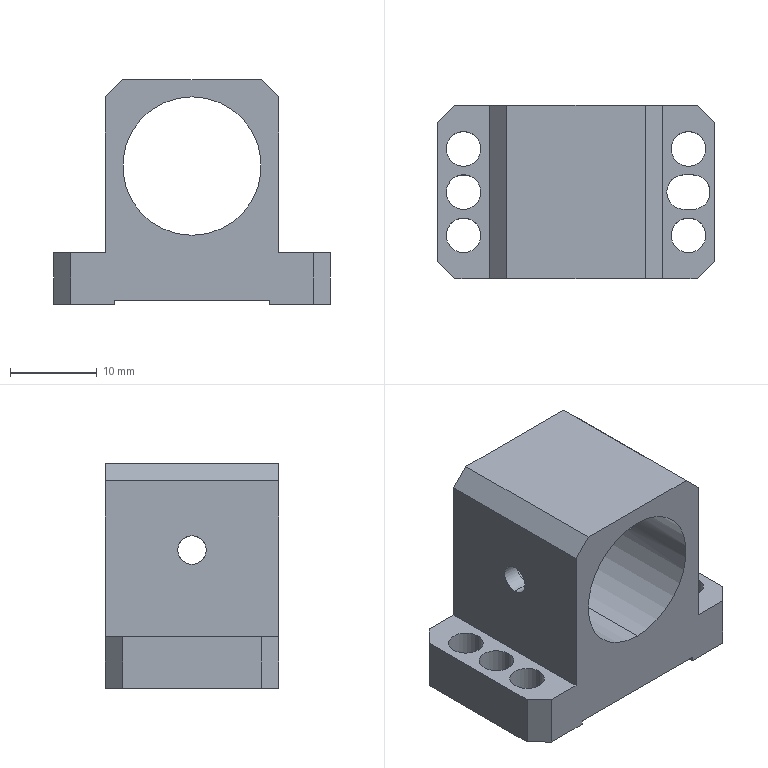NC program | NX | posted with a generic post | part box 32 x 20 x 26 mm
Lines 1 to 2179 of 2593, first 1714 of 2167 lines:
N10 G17 G21 G94 G90
(FLOOR_WALL , TOOL : D10JING)
N12 T11 M6
N14 G54
N16 G17 G0 G90 X-17.997 Y-20. B0. C0. S9500 M3
N18 G43 Z30. H11
N20 Z3.
N22 G94 G1 Z0. F1250.
N24 Y-17.
N26 Y17.
N28 X-13.426
N30 Y-17.
N32 X-8.855
N34 Y17.
N36 X-4.284
N38 Y-17.
N40 X0.287
N42 Y17.
N44 X4.858
N46 Y-17.
N48 X9.429
N50 Y17.
N52 X14.
N54 Y-17.
N56 Y-20.
N58 Z3.
N60 G0 Z30.
N62 M5
(ZLEVEL_PROFILE , TOOL : D10)
N64 T10 M6
N66 G54
N68 G17 G0 G90 X13.531 Y15.1 B0. C0. S9500 M3
N70 G43 Z30. H10
N72 Z1.5
N74 G94 G1 X14.32 Z1.459 F1000.
N76 X15.153 Y14.978 Z1.415
N78 X15.956 Y14.721 Z1.37
N80 X16.705 Y14.336 Z1.326
N82 X17.38 Y13.832 Z1.282
N84 X19.832 Y11.38 Z1.1
N86 X20.336 Y10.705 Z1.056
N88 X20.721 Y9.956 Z1.012
N90 X20.978 Y9.153 Z0.968
N92 X21.1 Y8.32 Z0.924
N94 Y-8.32 Z0.052
N96 X20.978 Y-9.153 Z0.008
N98 X20.721 Y-9.956 Z-0.037
N100 X20.336 Y-10.705 Z-0.081
N102 X19.832 Y-11.38 Z-0.125
N104 X17.38 Y-13.832 Z-0.307
N106 X16.705 Y-14.336 Z-0.351
N108 X15.956 Y-14.721 Z-0.395
N110 X15.153 Y-14.978 Z-0.439
N112 X14.32 Y-15.1 Z-0.483
N114 X14. Z-0.5
N116 X-14. F3000.
N118 G2 X-17.606 Y-13.606 R5.1
N120 G1 X-19.606 Y-11.606
N122 G2 X-21.1 Y-8. R5.1
N124 G1 Y8.
N126 G2 X-19.606 Y11.606 R5.1
N128 G1 X-17.606 Y13.606
N130 G2 X-14. Y15.1 R5.1
N132 G1 X14.
N134 G2 X17.606 Y13.606 R5.1
N136 G1 X19.606 Y11.606
N138 G2 X21.1 Y8. R5.1
N140 G1 Y-8.
N142 G2 X19.606 Y-11.606 R5.1
N144 G1 X17.606 Y-13.606
N146 G2 X14. Y-15.1 R5.1
N148 G1 X-13.764 Z-0.985
N150 X-13.984 Z-0.988
N152 X-14.204 Y-15.096 Z-0.992
N154 X-14.424 Y-15.082 Z-0.996
N156 X-14.643 Y-15.059 Z-1.
N158 G2 X-17.606 Y-13.606 R5.1
N160 G1 X-19.606 Y-11.606
N162 G2 X-21.1 Y-8. R5.1
N164 G1 Y8.
N166 G2 X-19.606 Y11.606 R5.1
N168 G1 X-17.606 Y13.606
N170 G2 X-14. Y15.1 R5.1
N172 G1 X14.
N174 G2 X17.606 Y13.606 R5.1
N176 G1 X19.606 Y11.606
N178 G2 X21.1 Y8. R5.1
N180 G1 Y-8.
N182 G2 X19.606 Y-11.606 R5.1
N184 G1 X17.606 Y-13.606
N186 G2 X14. Y-15.1 R5.1
N188 G1 X-13.764 Z-1.485
N190 X-13.984 Z-1.488
N192 X-14.204 Y-15.096 Z-1.492
N194 X-14.424 Y-15.082 Z-1.496
N196 X-14.643 Y-15.059 Z-1.5
N198 G2 X-17.606 Y-13.606 R5.1
N200 G1 X-19.606 Y-11.606
N202 G2 X-21.1 Y-8. R5.1
N204 G1 Y8.
N206 G2 X-19.606 Y11.606 R5.1
N208 G1 X-17.606 Y13.606
N210 G2 X-14. Y15.1 R5.1
N212 G1 X14.
N214 G2 X17.606 Y13.606 R5.1
N216 G1 X19.606 Y11.606
N218 G2 X21.1 Y8. R5.1
N220 G1 Y-8.
N222 G2 X19.606 Y-11.606 R5.1
N224 G1 X17.606 Y-13.606
N226 G2 X14. Y-15.1 R5.1
N228 G1 X-13.764 Z-1.985
N230 X-13.984 Z-1.988
N232 X-14.204 Y-15.096 Z-1.992
N234 X-14.424 Y-15.082 Z-1.996
N236 X-14.643 Y-15.059 Z-2.
N238 G2 X-17.606 Y-13.606 R5.1
N240 G1 X-19.606 Y-11.606
N242 G2 X-21.1 Y-8. R5.1
N244 G1 Y8.
N246 G2 X-19.606 Y11.606 R5.1
N248 G1 X-17.606 Y13.606
N250 G2 X-14. Y15.1 R5.1
N252 G1 X14.
N254 G2 X17.606 Y13.606 R5.1
N256 G1 X19.606 Y11.606
N258 G2 X21.1 Y8. R5.1
N260 G1 Y-8.
N262 G2 X19.606 Y-11.606 R5.1
N264 G1 X17.606 Y-13.606
N266 G2 X14. Y-15.1 R5.1
N268 G1 X-13.764 Z-2.485
N270 X-13.984 Z-2.488
N272 X-14.204 Y-15.096 Z-2.492
N274 X-14.424 Y-15.082 Z-2.496
N276 X-14.643 Y-15.059 Z-2.5
N278 G2 X-17.606 Y-13.606 R5.1
N280 G1 X-19.606 Y-11.606
N282 G2 X-21.1 Y-8. R5.1
N284 G1 Y8.
N286 G2 X-19.606 Y11.606 R5.1
N288 G1 X-17.606 Y13.606
N290 G2 X-14. Y15.1 R5.1
N292 G1 X14.
N294 G2 X17.606 Y13.606 R5.1
N296 G1 X19.606 Y11.606
N298 G2 X21.1 Y8. R5.1
N300 G1 Y-8.
N302 G2 X19.606 Y-11.606 R5.1
N304 G1 X17.606 Y-13.606
N306 G2 X14. Y-15.1 R5.1
N308 G1 X-13.764 Z-2.985
N310 X-13.984 Z-2.988
N312 X-14.204 Y-15.096 Z-2.992
N314 X-14.424 Y-15.082 Z-2.996
N316 X-14.643 Y-15.059 Z-3.
N318 G2 X-17.606 Y-13.606 R5.1
N320 G1 X-19.606 Y-11.606
N322 G2 X-21.1 Y-8. R5.1
N324 G1 Y8.
N326 G2 X-19.606 Y11.606 R5.1
N328 G1 X-17.606 Y13.606
N330 G2 X-14. Y15.1 R5.1
N332 G1 X14.
N334 G2 X17.606 Y13.606 R5.1
N336 G1 X19.606 Y11.606
N338 G2 X21.1 Y8. R5.1
N340 G1 Y-8.
N342 G2 X19.606 Y-11.606 R5.1
N344 G1 X17.606 Y-13.606
N346 G2 X14. Y-15.1 R5.1
N348 G1 X-13.764 Z-3.485
N350 X-13.984 Z-3.488
N352 X-14.204 Y-15.096 Z-3.492
N354 X-14.424 Y-15.082 Z-3.496
N356 X-14.643 Y-15.059 Z-3.5
N358 G2 X-17.606 Y-13.606 R5.1
N360 G1 X-19.606 Y-11.606
N362 G2 X-21.1 Y-8. R5.1
N364 G1 Y8.
N366 G2 X-19.606 Y11.606 R5.1
N368 G1 X-17.606 Y13.606
N370 G2 X-14. Y15.1 R5.1
N372 G1 X14.
N374 G2 X17.606 Y13.606 R5.1
N376 G1 X19.606 Y11.606
N378 G2 X21.1 Y8. R5.1
N380 G1 Y-8.
N382 G2 X19.606 Y-11.606 R5.1
N384 G1 X17.606 Y-13.606
N386 G2 X14. Y-15.1 R5.1
N388 G1 X-13.764 Z-3.985
N390 X-13.984 Z-3.988
N392 X-14.204 Y-15.096 Z-3.992
N394 X-14.424 Y-15.082 Z-3.996
N396 X-14.643 Y-15.059 Z-4.
N398 G2 X-17.606 Y-13.606 R5.1
N400 G1 X-19.606 Y-11.606
N402 G2 X-21.1 Y-8. R5.1
N404 G1 Y8.
N406 G2 X-19.606 Y11.606 R5.1
N408 G1 X-17.606 Y13.606
N410 G2 X-14. Y15.1 R5.1
N412 G1 X14.
N414 G2 X17.606 Y13.606 R5.1
N416 G1 X19.606 Y11.606
N418 G2 X21.1 Y8. R5.1
N420 G1 Y-8.
N422 G2 X19.606 Y-11.606 R5.1
N424 G1 X17.606 Y-13.606
N426 G2 X14. Y-15.1 R5.1
N428 G1 X-13.764 Z-4.485
N430 X-13.984 Z-4.488
N432 X-14.204 Y-15.096 Z-4.492
N434 X-14.424 Y-15.082 Z-4.496
N436 X-14.643 Y-15.059 Z-4.5
N438 G2 X-17.606 Y-13.606 R5.1
N440 G1 X-19.606 Y-11.606
N442 G2 X-21.1 Y-8. R5.1
N444 G1 Y8.
N446 G2 X-19.606 Y11.606 R5.1
N448 G1 X-17.606 Y13.606
N450 G2 X-14. Y15.1 R5.1
N452 G1 X14.
N454 G2 X17.606 Y13.606 R5.1
N456 G1 X19.606 Y11.606
N458 G2 X21.1 Y8. R5.1
N460 G1 Y-8.
N462 G2 X19.606 Y-11.606 R5.1
N464 G1 X17.606 Y-13.606
N466 G2 X14. Y-15.1 R5.1
N468 G1 X-13.764 Z-4.985
N470 X-13.984 Z-4.988
N472 X-14.204 Y-15.096 Z-4.992
N474 X-14.424 Y-15.082 Z-4.996
N476 X-14.643 Y-15.059 Z-5.
N478 G2 X-17.606 Y-13.606 R5.1
N480 G1 X-19.606 Y-11.606
N482 G2 X-21.1 Y-8. R5.1
N484 G1 Y8.
N486 G2 X-19.606 Y11.606 R5.1
N488 G1 X-17.606 Y13.606
N490 G2 X-14. Y15.1 R5.1
N492 G1 X14.
N494 G2 X17.606 Y13.606 R5.1
N496 G1 X19.606 Y11.606
N498 G2 X21.1 Y8. R5.1
N500 G1 Y-8.
N502 G2 X19.606 Y-11.606 R5.1
N504 G1 X17.606 Y-13.606
N506 G2 X14. Y-15.1 R5.1
N508 G1 X-13.764 Z-5.485
N510 X-13.984 Z-5.488
N512 X-14.204 Y-15.096 Z-5.492
N514 X-14.424 Y-15.082 Z-5.496
N516 X-14.643 Y-15.059 Z-5.5
N518 G2 X-17.606 Y-13.606 R5.1
N520 G1 X-19.606 Y-11.606
N522 G2 X-21.1 Y-8. R5.1
N524 G1 Y8.
N526 G2 X-19.606 Y11.606 R5.1
N528 G1 X-17.606 Y13.606
N530 G2 X-14. Y15.1 R5.1
N532 G1 X14.
N534 G2 X17.606 Y13.606 R5.1
N536 G1 X19.606 Y11.606
N538 G2 X21.1 Y8. R5.1
N540 G1 Y-8.
N542 G2 X19.606 Y-11.606 R5.1
N544 G1 X17.606 Y-13.606
N546 G2 X14. Y-15.1 R5.1
N548 G1 X-13.764 Z-5.985
N550 X-13.984 Z-5.988
N552 X-14.204 Y-15.096 Z-5.992
N554 X-14.424 Y-15.082 Z-5.996
N556 X-14.643 Y-15.059 Z-6.
N558 G2 X-17.606 Y-13.606 R5.1
N560 G1 X-19.606 Y-11.606
N562 G2 X-21.1 Y-8. R5.1
N564 G1 Y8.
N566 G2 X-19.606 Y11.606 R5.1
N568 G1 X-17.606 Y13.606
N570 G2 X-14. Y15.1 R5.1
N572 G1 X14.
N574 G2 X17.606 Y13.606 R5.1
N576 G1 X19.606 Y11.606
N578 G2 X21.1 Y8. R5.1
N580 G1 Y-8.
N582 G2 X19.606 Y-11.606 R5.1
N584 G1 X17.606 Y-13.606
N586 G2 X14. Y-15.1 R5.1
N588 G1 X-13.764 Z-6.485
N590 X-13.984 Z-6.488
N592 X-14.204 Y-15.096 Z-6.492
N594 X-14.424 Y-15.082 Z-6.496
N596 X-14.643 Y-15.059 Z-6.5
N598 G2 X-17.606 Y-13.606 R5.1
N600 G1 X-19.606 Y-11.606
N602 G2 X-21.1 Y-8. R5.1
N604 G1 Y8.
N606 G2 X-19.606 Y11.606 R5.1
N608 G1 X-17.606 Y13.606
N610 G2 X-14. Y15.1 R5.1
N612 G1 X14.
N614 G2 X17.606 Y13.606 R5.1
N616 G1 X19.606 Y11.606
N618 G2 X21.1 Y8. R5.1
N620 G1 Y-8.
N622 G2 X19.606 Y-11.606 R5.1
N624 G1 X17.606 Y-13.606
N626 G2 X14. Y-15.1 R5.1
N628 G1 X-13.764 Z-6.985
N630 X-13.984 Z-6.988
N632 X-14.204 Y-15.096 Z-6.992
N634 X-14.424 Y-15.082 Z-6.996
N636 X-14.643 Y-15.059 Z-7.
N638 G2 X-17.606 Y-13.606 R5.1
N640 G1 X-19.606 Y-11.606
N642 G2 X-21.1 Y-8. R5.1
N644 G1 Y8.
N646 G2 X-19.606 Y11.606 R5.1
N648 G1 X-17.606 Y13.606
N650 G2 X-14. Y15.1 R5.1
N652 G1 X14.
N654 G2 X17.606 Y13.606 R5.1
N656 G1 X19.606 Y11.606
N658 G2 X21.1 Y8. R5.1
N660 G1 Y-8.
N662 G2 X19.606 Y-11.606 R5.1
N664 G1 X17.606 Y-13.606
N666 G2 X14. Y-15.1 R5.1
N668 G1 X-13.764 Z-7.485
N670 X-13.984 Z-7.488
N672 X-14.204 Y-15.096 Z-7.492
N674 X-14.424 Y-15.082 Z-7.496
N676 X-14.643 Y-15.059 Z-7.5
N678 G2 X-17.606 Y-13.606 R5.1
N680 G1 X-19.606 Y-11.606
N682 G2 X-21.1 Y-8. R5.1
N684 G1 Y8.
N686 G2 X-19.606 Y11.606 R5.1
N688 G1 X-17.606 Y13.606
N690 G2 X-14. Y15.1 R5.1
N692 G1 X14.
N694 G2 X17.606 Y13.606 R5.1
N696 G1 X19.606 Y11.606
N698 G2 X21.1 Y8. R5.1
N700 G1 Y-8.
N702 G2 X19.606 Y-11.606 R5.1
N704 G1 X17.606 Y-13.606
N706 G2 X14. Y-15.1 R5.1
N708 G1 X-13.764 Z-7.985
N710 X-13.984 Z-7.988
N712 X-14.204 Y-15.096 Z-7.992
N714 X-14.424 Y-15.082 Z-7.996
N716 X-14.643 Y-15.059 Z-8.
N718 G2 X-17.606 Y-13.606 R5.1
N720 G1 X-19.606 Y-11.606
N722 G2 X-21.1 Y-8. R5.1
N724 G1 Y8.
N726 G2 X-19.606 Y11.606 R5.1
N728 G1 X-17.606 Y13.606
N730 G2 X-14. Y15.1 R5.1
N732 G1 X14.
N734 G2 X17.606 Y13.606 R5.1
N736 G1 X19.606 Y11.606
N738 G2 X21.1 Y8. R5.1
N740 G1 Y-8.
N742 G2 X19.606 Y-11.606 R5.1
N744 G1 X17.606 Y-13.606
N746 G2 X14. Y-15.1 R5.1
N748 G1 X-13.764 Z-8.485
N750 X-13.984 Z-8.488
N752 X-14.204 Y-15.096 Z-8.492
N754 X-14.424 Y-15.082 Z-8.496
N756 X-14.643 Y-15.059 Z-8.5
N758 G2 X-17.606 Y-13.606 R5.1
N760 G1 X-19.606 Y-11.606
N762 G2 X-21.1 Y-8. R5.1
N764 G1 Y8.
N766 G2 X-19.606 Y11.606 R5.1
N768 G1 X-17.606 Y13.606
N770 G2 X-14. Y15.1 R5.1
N772 G1 X14.
N774 G2 X17.606 Y13.606 R5.1
N776 G1 X19.606 Y11.606
N778 G2 X21.1 Y8. R5.1
N780 G1 Y-8.
N782 G2 X19.606 Y-11.606 R5.1
N784 G1 X17.606 Y-13.606
N786 G2 X14. Y-15.1 R5.1
N788 G1 X-13.764 Z-8.985
N790 X-13.984 Z-8.988
N792 X-14.204 Y-15.096 Z-8.992
N794 X-14.424 Y-15.082 Z-8.996
N796 X-14.643 Y-15.059 Z-9.
N798 G2 X-17.606 Y-13.606 R5.1
N800 G1 X-19.606 Y-11.606
N802 G2 X-21.1 Y-8. R5.1
N804 G1 Y8.
N806 G2 X-19.606 Y11.606 R5.1
N808 G1 X-17.606 Y13.606
N810 G2 X-14. Y15.1 R5.1
N812 G1 X14.
N814 G2 X17.606 Y13.606 R5.1
N816 G1 X19.606 Y11.606
N818 G2 X21.1 Y8. R5.1
N820 G1 Y-8.
N822 G2 X19.606 Y-11.606 R5.1
N824 G1 X17.606 Y-13.606
N826 G2 X14. Y-15.1 R5.1
N828 G1 X-13.764 Z-9.485
N830 X-13.984 Z-9.488
N832 X-14.204 Y-15.096 Z-9.492
N834 X-14.424 Y-15.082 Z-9.496
N836 X-14.643 Y-15.059 Z-9.5
N838 G2 X-17.606 Y-13.606 R5.1
N840 G1 X-19.606 Y-11.606
N842 G2 X-21.1 Y-8. R5.1
N844 G1 Y8.
N846 G2 X-19.606 Y11.606 R5.1
N848 G1 X-17.606 Y13.606
N850 G2 X-14. Y15.1 R5.1
N852 G1 X14.
N854 G2 X17.606 Y13.606 R5.1
N856 G1 X19.606 Y11.606
N858 G2 X21.1 Y8. R5.1
N860 G1 Y-8.
N862 G2 X19.606 Y-11.606 R5.1
N864 G1 X17.606 Y-13.606
N866 G2 X14. Y-15.1 R5.1
N868 G1 X-13.764 Z-9.985
N870 X-13.984 Z-9.988
N872 X-14.204 Y-15.096 Z-9.992
N874 X-14.424 Y-15.082 Z-9.996
N876 X-14.643 Y-15.059 Z-10.
N878 G2 X-17.606 Y-13.606 R5.1
N880 G1 X-19.606 Y-11.606
N882 G2 X-21.1 Y-8. R5.1
N884 G1 Y8.
N886 G2 X-19.606 Y11.606 R5.1
N888 G1 X-17.606 Y13.606
N890 G2 X-14. Y15.1 R5.1
N892 G1 X14.
N894 G2 X17.606 Y13.606 R5.1
N896 G1 X19.606 Y11.606
N898 G2 X21.1 Y8. R5.1
N900 G1 Y-8.
N902 G2 X19.606 Y-11.606 R5.1
N904 G1 X17.606 Y-13.606
N906 G2 X14. Y-15.1 R5.1
N908 G1 X-13.764 Z-10.485
N910 X-13.984 Z-10.488
N912 X-14.204 Y-15.096 Z-10.492
N914 X-14.424 Y-15.082 Z-10.496
N916 X-14.643 Y-15.059 Z-10.5
N918 G2 X-17.606 Y-13.606 R5.1
N920 G1 X-19.606 Y-11.606
N922 G2 X-21.1 Y-8. R5.1
N924 G1 Y8.
N926 G2 X-19.606 Y11.606 R5.1
N928 G1 X-17.606 Y13.606
N930 G2 X-14. Y15.1 R5.1
N932 G1 X14.
N934 G2 X17.606 Y13.606 R5.1
N936 G1 X19.606 Y11.606
N938 G2 X21.1 Y8. R5.1
N940 G1 Y-8.
N942 G2 X19.606 Y-11.606 R5.1
N944 G1 X17.606 Y-13.606
N946 G2 X14. Y-15.1 R5.1
N948 G1 X-13.764 Z-10.985
N950 X-13.984 Z-10.988
N952 X-14.204 Y-15.096 Z-10.992
N954 X-14.424 Y-15.082 Z-10.996
N956 X-14.643 Y-15.059 Z-11.
N958 G2 X-17.606 Y-13.606 R5.1
N960 G1 X-19.606 Y-11.606
N962 G2 X-21.1 Y-8. R5.1
N964 G1 Y8.
N966 G2 X-19.606 Y11.606 R5.1
N968 G1 X-17.606 Y13.606
N970 G2 X-14. Y15.1 R5.1
N972 G1 X14.
N974 G2 X17.606 Y13.606 R5.1
N976 G1 X19.606 Y11.606
N978 G2 X21.1 Y8. R5.1
N980 G1 Y-8.
N982 G2 X19.606 Y-11.606 R5.1
N984 G1 X17.606 Y-13.606
N986 G2 X14. Y-15.1 R5.1
N988 G1 X-13.764 Z-11.485
N990 X-13.984 Z-11.488
N992 X-14.204 Y-15.096 Z-11.492
N994 X-14.424 Y-15.082 Z-11.496
N996 X-14.643 Y-15.059 Z-11.5
N998 G2 X-17.606 Y-13.606 R5.1
N1000 G1 X-19.606 Y-11.606
N1002 G2 X-21.1 Y-8. R5.1
N1004 G1 Y8.
N1006 G2 X-19.606 Y11.606 R5.1
N1008 G1 X-17.606 Y13.606
N1010 G2 X-14. Y15.1 R5.1
N1012 G1 X14.
N1014 G2 X17.606 Y13.606 R5.1
N1016 G1 X19.606 Y11.606
N1018 G2 X21.1 Y8. R5.1
N1020 G1 Y-8.
N1022 G2 X19.606 Y-11.606 R5.1
N1024 G1 X17.606 Y-13.606
N1026 G2 X14. Y-15.1 R5.1
N1028 G1 X-13.764 Z-11.985
N1030 X-13.984 Z-11.988
N1032 X-14.204 Y-15.096 Z-11.992
N1034 X-14.424 Y-15.082 Z-11.996
N1036 X-14.643 Y-15.059 Z-12.
N1038 G2 X-17.606 Y-13.606 R5.1
N1040 G1 X-19.606 Y-11.606
N1042 G2 X-21.1 Y-8. R5.1
N1044 G1 Y8.
N1046 G2 X-19.606 Y11.606 R5.1
N1048 G1 X-17.606 Y13.606
N1050 G2 X-14. Y15.1 R5.1
N1052 G1 X14.
N1054 G2 X17.606 Y13.606 R5.1
N1056 G1 X19.606 Y11.606
N1058 G2 X21.1 Y8. R5.1
N1060 G1 Y-8.
N1062 G2 X19.606 Y-11.606 R5.1
N1064 G1 X17.606 Y-13.606
N1066 G2 X14. Y-15.1 R5.1
N1068 G1 X-13.764 Z-12.485
N1070 X-13.984 Z-12.488
N1072 X-14.204 Y-15.096 Z-12.492
N1074 X-14.424 Y-15.082 Z-12.496
N1076 X-14.643 Y-15.059 Z-12.5
N1078 G2 X-17.606 Y-13.606 R5.1
N1080 G1 X-19.606 Y-11.606
N1082 G2 X-21.1 Y-8. R5.1
N1084 G1 Y8.
N1086 G2 X-19.606 Y11.606 R5.1
N1088 G1 X-17.606 Y13.606
N1090 G2 X-14. Y15.1 R5.1
N1092 G1 X14.
N1094 G2 X17.606 Y13.606 R5.1
N1096 G1 X19.606 Y11.606
N1098 G2 X21.1 Y8. R5.1
N1100 G1 Y-8.
N1102 G2 X19.606 Y-11.606 R5.1
N1104 G1 X17.606 Y-13.606
N1106 G2 X14. Y-15.1 R5.1
N1108 G1 X-13.764 Z-12.985
N1110 X-13.984 Z-12.988
N1112 X-14.204 Y-15.096 Z-12.992
N1114 X-14.424 Y-15.082 Z-12.996
N1116 X-14.643 Y-15.059 Z-13.
N1118 G2 X-17.606 Y-13.606 R5.1
N1120 G1 X-19.606 Y-11.606
N1122 G2 X-21.1 Y-8. R5.1
N1124 G1 Y8.
N1126 G2 X-19.606 Y11.606 R5.1
N1128 G1 X-17.606 Y13.606
N1130 G2 X-14. Y15.1 R5.1
N1132 G1 X14.
N1134 G2 X17.606 Y13.606 R5.1
N1136 G1 X19.606 Y11.606
N1138 G2 X21.1 Y8. R5.1
N1140 G1 Y-8.
N1142 G2 X19.606 Y-11.606 R5.1
N1144 G1 X17.606 Y-13.606
N1146 G2 X14. Y-15.1 R5.1
N1148 G1 X-13.764 Z-13.485
N1150 X-13.984 Z-13.488
N1152 X-14.204 Y-15.096 Z-13.492
N1154 X-14.424 Y-15.082 Z-13.496
N1156 X-14.643 Y-15.059 Z-13.5
N1158 G2 X-17.606 Y-13.606 R5.1
N1160 G1 X-19.606 Y-11.606
N1162 G2 X-21.1 Y-8. R5.1
N1164 G1 Y8.
N1166 G2 X-19.606 Y11.606 R5.1
N1168 G1 X-17.606 Y13.606
N1170 G2 X-14. Y15.1 R5.1
N1172 G1 X14.
N1174 G2 X17.606 Y13.606 R5.1
N1176 G1 X19.606 Y11.606
N1178 G2 X21.1 Y8. R5.1
N1180 G1 Y-8.
N1182 G2 X19.606 Y-11.606 R5.1
N1184 G1 X17.606 Y-13.606
N1186 G2 X14. Y-15.1 R5.1
N1188 G1 X-13.764 Z-13.985
N1190 X-13.984 Z-13.988
N1192 X-14.204 Y-15.096 Z-13.992
N1194 X-14.424 Y-15.082 Z-13.996
N1196 X-14.643 Y-15.059 Z-14.
N1198 G2 X-17.606 Y-13.606 R5.1
N1200 G1 X-19.606 Y-11.606
N1202 G2 X-21.1 Y-8. R5.1
N1204 G1 Y8.
N1206 G2 X-19.606 Y11.606 R5.1
N1208 G1 X-17.606 Y13.606
N1210 G2 X-14. Y15.1 R5.1
N1212 G1 X14.
N1214 G2 X17.606 Y13.606 R5.1
N1216 G1 X19.606 Y11.606
N1218 G2 X21.1 Y8. R5.1
N1220 G1 Y-8.
N1222 G2 X19.606 Y-11.606 R5.1
N1224 G1 X17.606 Y-13.606
N1226 G2 X14. Y-15.1 R5.1
N1228 G1 X-13.764 Z-14.485
N1230 X-13.984 Z-14.488
N1232 X-14.204 Y-15.096 Z-14.492
N1234 X-14.424 Y-15.082 Z-14.496
N1236 X-14.643 Y-15.059 Z-14.5
N1238 G2 X-17.606 Y-13.606 R5.1
N1240 G1 X-19.606 Y-11.606
N1242 G2 X-21.1 Y-8. R5.1
N1244 G1 Y8.
N1246 G2 X-19.606 Y11.606 R5.1
N1248 G1 X-17.606 Y13.606
N1250 G2 X-14. Y15.1 R5.1
N1252 G1 X14.
N1254 G2 X17.606 Y13.606 R5.1
N1256 G1 X19.606 Y11.606
N1258 G2 X21.1 Y8. R5.1
N1260 G1 Y-8.
N1262 G2 X19.606 Y-11.606 R5.1
N1264 G1 X17.606 Y-13.606
N1266 G2 X14. Y-15.1 R5.1
N1268 G1 X-13.764 Z-14.985
N1270 X-13.984 Z-14.988
N1272 X-14.204 Y-15.096 Z-14.992
N1274 X-14.424 Y-15.082 Z-14.996
N1276 X-14.643 Y-15.059 Z-15.
N1278 G2 X-17.606 Y-13.606 R5.1
N1280 G1 X-19.606 Y-11.606
N1282 G2 X-21.1 Y-8. R5.1
N1284 G1 Y8.
N1286 G2 X-19.606 Y11.606 R5.1
N1288 G1 X-17.606 Y13.606
N1290 G2 X-14. Y15.1 R5.1
N1292 G1 X14.
N1294 G2 X17.606 Y13.606 R5.1
N1296 G1 X19.606 Y11.606
N1298 G2 X21.1 Y8. R5.1
N1300 G1 Y-8.
N1302 G2 X19.606 Y-11.606 R5.1
N1304 G1 X17.606 Y-13.606
N1306 G2 X14. Y-15.1 R5.1
N1308 G1 X-13.764 Z-15.485
N1310 X-13.984 Z-15.488
N1312 X-14.204 Y-15.096 Z-15.492
N1314 X-14.424 Y-15.082 Z-15.496
N1316 X-14.643 Y-15.059 Z-15.5
N1318 G2 X-17.606 Y-13.606 R5.1
N1320 G1 X-19.606 Y-11.606
N1322 G2 X-21.1 Y-8. R5.1
N1324 G1 Y8.
N1326 G2 X-19.606 Y11.606 R5.1
N1328 G1 X-17.606 Y13.606
N1330 G2 X-14. Y15.1 R5.1
N1332 G1 X14.
N1334 G2 X17.606 Y13.606 R5.1
N1336 G1 X19.606 Y11.606
N1338 G2 X21.1 Y8. R5.1
N1340 G1 Y-8.
N1342 G2 X19.606 Y-11.606 R5.1
N1344 G1 X17.606 Y-13.606
N1346 G2 X14. Y-15.1 R5.1
N1348 G1 X-13.764 Z-15.985
N1350 X-13.984 Z-15.988
N1352 X-14.204 Y-15.096 Z-15.992
N1354 X-14.424 Y-15.082 Z-15.996
N1356 X-14.643 Y-15.059 Z-16.
N1358 G2 X-17.606 Y-13.606 R5.1
N1360 G1 X-19.606 Y-11.606
N1362 G2 X-21.1 Y-8. R5.1
N1364 G1 Y8.
N1366 G2 X-19.606 Y11.606 R5.1
N1368 G1 X-17.606 Y13.606
N1370 G2 X-14. Y15.1 R5.1
N1372 G1 X14.
N1374 G2 X17.606 Y13.606 R5.1
N1376 G1 X19.606 Y11.606
N1378 G2 X21.1 Y8. R5.1
N1380 G1 Y-8.
N1382 G2 X19.606 Y-11.606 R5.1
N1384 G1 X17.606 Y-13.606
N1386 G2 X14. Y-15.1 R5.1
N1388 G1 X-13.764 Z-16.485
N1390 X-13.984 Z-16.488
N1392 X-14.204 Y-15.096 Z-16.492
N1394 X-14.424 Y-15.082 Z-16.496
N1396 X-14.643 Y-15.059 Z-16.5
N1398 G2 X-17.606 Y-13.606 R5.1
N1400 G1 X-19.606 Y-11.606
N1402 G2 X-21.1 Y-8. R5.1
N1404 G1 Y8.
N1406 G2 X-19.606 Y11.606 R5.1
N1408 G1 X-17.606 Y13.606
N1410 G2 X-14. Y15.1 R5.1
N1412 G1 X14.
N1414 G2 X17.606 Y13.606 R5.1
N1416 G1 X19.606 Y11.606
N1418 G2 X21.1 Y8. R5.1
N1420 G1 Y-8.
N1422 G2 X19.606 Y-11.606 R5.1
N1424 G1 X17.606 Y-13.606
N1426 G2 X14. Y-15.1 R5.1
N1428 G1 X-13.764 Z-16.985
N1430 X-13.984 Z-16.988
N1432 X-14.204 Y-15.096 Z-16.992
N1434 X-14.424 Y-15.082 Z-16.996
N1436 X-14.643 Y-15.059 Z-17.
N1438 G2 X-17.606 Y-13.606 R5.1
N1440 G1 X-19.606 Y-11.606
N1442 G2 X-21.1 Y-8. R5.1
N1444 G1 Y8.
N1446 G2 X-19.606 Y11.606 R5.1
N1448 G1 X-17.606 Y13.606
N1450 G2 X-14. Y15.1 R5.1
N1452 G1 X14.
N1454 G2 X17.606 Y13.606 R5.1
N1456 G1 X19.606 Y11.606
N1458 G2 X21.1 Y8. R5.1
N1460 G1 Y-8.
N1462 G2 X19.606 Y-11.606 R5.1
N1464 G1 X17.606 Y-13.606
N1466 G2 X14. Y-15.1 R5.1
N1468 G1 X-13.764 Z-17.485
N1470 X-13.984 Z-17.488
N1472 X-14.204 Y-15.096 Z-17.492
N1474 X-14.424 Y-15.082 Z-17.496
N1476 X-14.643 Y-15.059 Z-17.5
N1478 G2 X-17.606 Y-13.606 R5.1
N1480 G1 X-19.606 Y-11.606
N1482 G2 X-21.1 Y-8. R5.1
N1484 G1 Y8.
N1486 G2 X-19.606 Y11.606 R5.1
N1488 G1 X-17.606 Y13.606
N1490 G2 X-14. Y15.1 R5.1
N1492 G1 X14.
N1494 G2 X17.606 Y13.606 R5.1
N1496 G1 X19.606 Y11.606
N1498 G2 X21.1 Y8. R5.1
N1500 G1 Y-8.
N1502 G2 X19.606 Y-11.606 R5.1
N1504 G1 X17.606 Y-13.606
N1506 G2 X14. Y-15.1 R5.1
N1508 G1 X-13.764 Z-17.985
N1510 X-13.984 Z-17.988
N1512 X-14.204 Y-15.096 Z-17.992
N1514 X-14.424 Y-15.082 Z-17.996
N1516 X-14.643 Y-15.059 Z-18.
N1518 G2 X-17.606 Y-13.606 R5.1
N1520 G1 X-19.606 Y-11.606
N1522 G2 X-21.1 Y-8. R5.1
N1524 G1 Y8.
N1526 G2 X-19.606 Y11.606 R5.1
N1528 G1 X-17.606 Y13.606
N1530 G2 X-14. Y15.1 R5.1
N1532 G1 X14.
N1534 G2 X17.606 Y13.606 R5.1
N1536 G1 X19.606 Y11.606
N1538 G2 X21.1 Y8. R5.1
N1540 G1 Y-8.
N1542 G2 X19.606 Y-11.606 R5.1
N1544 G1 X17.606 Y-13.606
N1546 G2 X14. Y-15.1 R5.1
N1548 G1 X-13.764 Z-18.485
N1550 X-13.984 Z-18.488
N1552 X-14.204 Y-15.096 Z-18.492
N1554 X-14.424 Y-15.082 Z-18.496
N1556 X-14.643 Y-15.059 Z-18.5
N1558 G2 X-17.606 Y-13.606 R5.1
N1560 G1 X-19.606 Y-11.606
N1562 G2 X-21.1 Y-8. R5.1
N1564 G1 Y8.
N1566 G2 X-19.606 Y11.606 R5.1
N1568 G1 X-17.606 Y13.606
N1570 G2 X-14. Y15.1 R5.1
N1572 G1 X14.
N1574 G2 X17.606 Y13.606 R5.1
N1576 G1 X19.606 Y11.606
N1578 G2 X21.1 Y8. R5.1
N1580 G1 Y-8.
N1582 G2 X19.606 Y-11.606 R5.1
N1584 G1 X17.606 Y-13.606
N1586 G2 X14. Y-15.1 R5.1
N1588 G1 X-13.764 Z-18.985
N1590 X-13.984 Z-18.988
N1592 X-14.204 Y-15.096 Z-18.992
N1594 X-14.424 Y-15.082 Z-18.996
N1596 X-14.643 Y-15.059 Z-19.
N1598 G2 X-17.606 Y-13.606 R5.1
N1600 G1 X-19.606 Y-11.606
N1602 G2 X-21.1 Y-8. R5.1
N1604 G1 Y8.
N1606 G2 X-19.606 Y11.606 R5.1
N1608 G1 X-17.606 Y13.606
N1610 G2 X-14. Y15.1 R5.1
N1612 G1 X14.
N1614 G2 X17.606 Y13.606 R5.1
N1616 G1 X19.606 Y11.606
N1618 G2 X21.1 Y8. R5.1
N1620 G1 Y-8.
N1622 G2 X19.606 Y-11.606 R5.1
N1624 G1 X17.606 Y-13.606
N1626 G2 X14. Y-15.1 R5.1
N1628 G1 X-13.764 Z-19.485
N1630 X-13.984 Z-19.488
N1632 X-14.204 Y-15.096 Z-19.492
N1634 X-14.424 Y-15.082 Z-19.496
N1636 X-14.643 Y-15.059 Z-19.5
N1638 G2 X-17.606 Y-13.606 R5.1
N1640 G1 X-19.606 Y-11.606
N1642 G2 X-21.1 Y-8. R5.1
N1644 G1 Y8.
N1646 G2 X-19.606 Y11.606 R5.1
N1648 G1 X-17.606 Y13.606
N1650 G2 X-14. Y15.1 R5.1
N1652 G1 X14.
N1654 G2 X17.606 Y13.606 R5.1
N1656 G1 X19.606 Y11.606
N1658 G2 X21.1 Y8. R5.1
N1660 G1 Y-8.
N1662 G2 X19.606 Y-11.606 R5.1
N1664 G1 X17.606 Y-13.606
N1666 G2 X14. Y-15.1 R5.1
N1668 G1 X-13.764 Z-19.985
N1670 X-13.984 Z-19.988
N1672 X-14.204 Y-15.096 Z-19.992
N1674 X-14.424 Y-15.082 Z-19.996
N1676 X-14.643 Y-15.059 Z-20.
N1678 G2 X-17.606 Y-13.606 R5.1
N1680 G1 X-19.606 Y-11.606
N1682 G2 X-21.1 Y-8. R5.1
N1684 G1 Y8.
N1686 G2 X-19.606 Y11.606 R5.1
N1688 G1 X-17.606 Y13.606
N1690 G2 X-14. Y15.1 R5.1
N1692 G1 X14.
N1694 G2 X17.606 Y13.606 R5.1
N1696 G1 X19.606 Y11.606
N1698 G2 X21.1 Y8. R5.1
N1700 G1 Y-8.
N1702 G2 X19.606 Y-11.606 R5.1
N1704 G1 X17.606 Y-13.606
N1706 G2 X14. Y-15.1 R5.1
N1708 G1 X-13.764 Z-20.485
N1710 X-13.984 Z-20.488
N1712 X-14.204 Y-15.096 Z-20.492
N1714 X-14.424 Y-15.082 Z-20.496
N1716 X-14.643 Y-15.059 Z-20.5
N1718 G2 X-17.606 Y-13.606 R5.1
N1720 G1 X-19.606 Y-11.606
N1722 G2 X-21.1 Y-8. R5.1
N1724 G1 Y8.
N1726 G2 X-19.606 Y11.606 R5.1
N1728 G1 X-17.606 Y13.606
N1730 G2 X-14. Y15.1 R5.1
N1732 G1 X14.
N1734 G2 X17.606 Y13.606 R5.1
N1736 G1 X19.606 Y11.606
N1738 G2 X21.1 Y8. R5.1
N1740 G1 Y-8.
N1742 G2 X19.606 Y-11.606 R5.1
N1744 G1 X17.606 Y-13.606
N1746 G2 X14. Y-15.1 R5.1
N1748 G1 X-13.764 Z-20.985
N1750 X-13.984 Z-20.988
N1752 X-14.204 Y-15.096 Z-20.992
N1754 X-14.424 Y-15.082 Z-20.996
N1756 X-14.643 Y-15.059 Z-21.
N1758 G2 X-17.606 Y-13.606 R5.1
N1760 G1 X-19.606 Y-11.606
N1762 G2 X-21.1 Y-8. R5.1
N1764 G1 Y8.
N1766 G2 X-19.606 Y11.606 R5.1
N1768 G1 X-17.606 Y13.606
N1770 G2 X-14. Y15.1 R5.1
N1772 G1 X14.
N1774 G2 X17.606 Y13.606 R5.1
N1776 G1 X19.606 Y11.606
N1778 G2 X21.1 Y8. R5.1
N1780 G1 Y-8.
N1782 G2 X19.606 Y-11.606 R5.1
N1784 G1 X17.606 Y-13.606
N1786 G2 X14. Y-15.1 R5.1
N1788 G1 X-13.764 Z-21.485
N1790 X-13.984 Z-21.488
N1792 X-14.204 Y-15.096 Z-21.492
N1794 X-14.424 Y-15.082 Z-21.496
N1796 X-14.643 Y-15.059 Z-21.5
N1798 G2 X-17.606 Y-13.606 R5.1
N1800 G1 X-19.606 Y-11.606
N1802 G2 X-21.1 Y-8. R5.1
N1804 G1 Y8.
N1806 G2 X-19.606 Y11.606 R5.1
N1808 G1 X-17.606 Y13.606
N1810 G2 X-14. Y15.1 R5.1
N1812 G1 X14.
N1814 G2 X17.606 Y13.606 R5.1
N1816 G1 X19.606 Y11.606
N1818 G2 X21.1 Y8. R5.1
N1820 G1 Y-8.
N1822 G2 X19.606 Y-11.606 R5.1
N1824 G1 X17.606 Y-13.606
N1826 G2 X14. Y-15.1 R5.1
N1828 G1 X-13.764 Z-21.985
N1830 X-13.984 Z-21.988
N1832 X-14.204 Y-15.096 Z-21.992
N1834 X-14.424 Y-15.082 Z-21.996
N1836 X-14.643 Y-15.059 Z-22.
N1838 G2 X-17.606 Y-13.606 R5.1
N1840 G1 X-19.606 Y-11.606
N1842 G2 X-21.1 Y-8. R5.1
N1844 G1 Y8.
N1846 G2 X-19.606 Y11.606 R5.1
N1848 G1 X-17.606 Y13.606
N1850 G2 X-14. Y15.1 R5.1
N1852 G1 X14.
N1854 G2 X17.606 Y13.606 R5.1
N1856 G1 X19.606 Y11.606
N1858 G2 X21.1 Y8. R5.1
N1860 G1 Y-8.
N1862 G2 X19.606 Y-11.606 R5.1
N1864 G1 X17.606 Y-13.606
N1866 G2 X14. Y-15.1 R5.1
N1868 G1 X-13.764 Z-22.485
N1870 X-13.984 Z-22.488
N1872 X-14.204 Y-15.096 Z-22.492
N1874 X-14.424 Y-15.082 Z-22.496
N1876 X-14.643 Y-15.059 Z-22.5
N1878 G2 X-17.606 Y-13.606 R5.1
N1880 G1 X-19.606 Y-11.606
N1882 G2 X-21.1 Y-8. R5.1
N1884 G1 Y8.
N1886 G2 X-19.606 Y11.606 R5.1
N1888 G1 X-17.606 Y13.606
N1890 G2 X-14. Y15.1 R5.1
N1892 G1 X14.
N1894 G2 X17.606 Y13.606 R5.1
N1896 G1 X19.606 Y11.606
N1898 G2 X21.1 Y8. R5.1
N1900 G1 Y-8.
N1902 G2 X19.606 Y-11.606 R5.1
N1904 G1 X17.606 Y-13.606
N1906 G2 X14. Y-15.1 R5.1
N1908 G1 X-13.764 Z-22.985
N1910 X-13.984 Z-22.988
N1912 X-14.204 Y-15.096 Z-22.992
N1914 X-14.424 Y-15.082 Z-22.996
N1916 X-14.643 Y-15.059 Z-23.
N1918 G2 X-17.606 Y-13.606 R5.1
N1920 G1 X-19.606 Y-11.606
N1922 G2 X-21.1 Y-8. R5.1
N1924 G1 Y8.
N1926 G2 X-19.606 Y11.606 R5.1
N1928 G1 X-17.606 Y13.606
N1930 G2 X-14. Y15.1 R5.1
N1932 G1 X14.
N1934 G2 X17.606 Y13.606 R5.1
N1936 G1 X19.606 Y11.606
N1938 G2 X21.1 Y8. R5.1
N1940 G1 Y-8.
N1942 G2 X19.606 Y-11.606 R5.1
N1944 G1 X17.606 Y-13.606
N1946 G2 X14. Y-15.1 R5.1
N1948 G1 X-13.764 Z-23.485
N1950 X-13.984 Z-23.488
N1952 X-14.204 Y-15.096 Z-23.492
N1954 X-14.424 Y-15.082 Z-23.496
N1956 X-14.643 Y-15.059 Z-23.5
N1958 G2 X-17.606 Y-13.606 R5.1
N1960 G1 X-19.606 Y-11.606
N1962 G2 X-21.1 Y-8. R5.1
N1964 G1 Y8.
N1966 G2 X-19.606 Y11.606 R5.1
N1968 G1 X-17.606 Y13.606
N1970 G2 X-14. Y15.1 R5.1
N1972 G1 X14.
N1974 G2 X17.606 Y13.606 R5.1
N1976 G1 X19.606 Y11.606
N1978 G2 X21.1 Y8. R5.1
N1980 G1 Y-8.
N1982 G2 X19.606 Y-11.606 R5.1
N1984 G1 X17.606 Y-13.606
N1986 G2 X14. Y-15.1 R5.1
N1988 G1 X-13.764 Z-23.985
N1990 X-13.984 Z-23.988
N1992 X-14.204 Y-15.096 Z-23.992
N1994 X-14.424 Y-15.082 Z-23.996
N1996 X-14.643 Y-15.059 Z-24.
N1998 G2 X-17.606 Y-13.606 R5.1
N2000 G1 X-19.606 Y-11.606
N2002 G2 X-21.1 Y-8. R5.1
N2004 G1 Y8.
N2006 G2 X-19.606 Y11.606 R5.1
N2008 G1 X-17.606 Y13.606
N2010 G2 X-14. Y15.1 R5.1
N2012 G1 X14.
N2014 G2 X17.606 Y13.606 R5.1
N2016 G1 X19.606 Y11.606
N2018 G2 X21.1 Y8. R5.1
N2020 G1 Y-8.
N2022 G2 X19.606 Y-11.606 R5.1
N2024 G1 X17.606 Y-13.606
N2026 G2 X14. Y-15.1 R5.1
N2028 G1 X-13.764 Z-24.485
N2030 X-13.984 Z-24.488
N2032 X-14.204 Y-15.096 Z-24.492
N2034 X-14.424 Y-15.082 Z-24.496
N2036 X-14.643 Y-15.059 Z-24.5
N2038 G2 X-17.606 Y-13.606 R5.1
N2040 G1 X-19.606 Y-11.606
N2042 G2 X-21.1 Y-8. R5.1
N2044 G1 Y8.
N2046 G2 X-19.606 Y11.606 R5.1
N2048 G1 X-17.606 Y13.606
N2050 G2 X-14. Y15.1 R5.1
N2052 G1 X14.
N2054 G2 X17.606 Y13.606 R5.1
N2056 G1 X19.606 Y11.606
N2058 G2 X21.1 Y8. R5.1
N2060 G1 Y-8.
N2062 G2 X19.606 Y-11.606 R5.1
N2064 G1 X17.606 Y-13.606
N2066 G2 X14. Y-15.1 R5.1
N2068 G1 X-13.764 Z-24.985
N2070 X-13.984 Z-24.988
N2072 X-14.204 Y-15.096 Z-24.992
N2074 X-14.424 Y-15.082 Z-24.996
N2076 X-14.643 Y-15.059 Z-25.
N2078 G2 X-17.606 Y-13.606 R5.1
N2080 G1 X-19.606 Y-11.606
N2082 G2 X-21.1 Y-8. R5.1
N2084 G1 Y8.
N2086 G2 X-19.606 Y11.606 R5.1
N2088 G1 X-17.606 Y13.606
N2090 G2 X-14. Y15.1 R5.1
N2092 G1 X14.
N2094 G2 X17.606 Y13.606 R5.1
N2096 G1 X19.606 Y11.606
N2098 G2 X21.1 Y8. R5.1
N2100 G1 Y-8.
N2102 G2 X19.606 Y-11.606 R5.1
N2104 G1 X17.606 Y-13.606
N2106 G2 X14. Y-15.1 R5.1
N2108 G1 X-13.764 Z-25.485
N2110 X-13.984 Z-25.488
N2112 X-14.204 Y-15.096 Z-25.492
N2114 X-14.424 Y-15.082 Z-25.496
N2116 X-14.643 Y-15.059 Z-25.5
N2118 G2 X-17.606 Y-13.606 R5.1
N2120 G1 X-19.606 Y-11.606
N2122 G2 X-21.1 Y-8. R5.1
N2124 G1 Y8.
N2126 G2 X-19.606 Y11.606 R5.1
N2128 G1 X-17.606 Y13.606
N2130 G2 X-14. Y15.1 R5.1
N2132 G1 X14.
N2134 G2 X17.606 Y13.606 R5.1
N2136 G1 X19.606 Y11.606
N2138 G2 X21.1 Y8. R5.1
N2140 G1 Y-8.
N2142 G2 X19.606 Y-11.606 R5.1
N2144 G1 X17.606 Y-13.606
N2146 G2 X14. Y-15.1 R5.1
N2148 G1 X-13.764 Z-25.985
N2150 X-13.984 Z-25.988
N2152 X-14.204 Y-15.096 Z-25.992
N2154 X-14.424 Y-15.082 Z-25.996
N2156 X-14.643 Y-15.059 Z-26.
N2158 G2 X-17.606 Y-13.606 R5.1
N2160 G1 X-19.606 Y-11.606
N2162 G2 X-21.1 Y-8. R5.1
N2164 G1 Y8.
N2166 G2 X-19.606 Y11.606 R5.1
N2168 G1 X-17.606 Y13.606
N2170 G2 X-14. Y15.1 R5.1
N2172 G1 X14.
N2174 G2 X17.606 Y13.606 R5.1
N2176 G1 X19.606 Y11.606
N2178 G2 X21.1 Y8. R5.1
N2180 G1 Y-8.
N2182 G2 X19.606 Y-11.606 R5.1
N2184 G1 X17.606 Y-13.606
N2186 G2 X14. Y-15.1 R5.1
N2188 G1 X-14.
N2190 G2 X-14.643 Y-15.059 R5.1
N2192 G1 Z-24.5
N2194 G0 Z30.
(FLOOR_WALL_1 , TOOL : D10)
N2196 X-22. Y-0.766
N2198 Z0.503
N2200 G1 Z-0.498 F1000.
N2202 X-16.357
N2204 G3 X-16. Y0. R1.
N2206 G1 Y8. F2500.
N2208 X-15.1 Y8.9
N2210 Y-8.9
N2212 X-16. Y-8.
N2214 Y0.
N2216 G3 X-16.357 Y0.766 R1.
N2218 G1 X-22.
N2220 Z0.503
N2222 G0 Y-0.766 Z0.005
N2224 G1 Z-0.995 F1000.
N2226 X-16.357
N2228 G3 X-16. Y0. R1.
N2230 G1 Y8. F2500.
N2232 X-15.1 Y8.9
N2234 Y-8.9
N2236 X-16. Y-8.
N2238 Y0.
N2240 G3 X-16.357 Y0.766 R1.
N2242 G1 X-22.
N2244 Z0.005
N2246 G0 Y-0.766 Z-0.493
N2248 G1 Z-1.493 F1000.
N2250 X-16.357
N2252 G3 X-16. Y0. R1.
N2254 G1 Y8. F2500.
N2256 X-15.1 Y8.9
N2258 Y-8.9
N2260 X-16. Y-8.
N2262 Y0.
N2264 G3 X-16.357 Y0.766 R1.
N2266 G1 X-22.
N2268 Z-0.493
N2270 G0 Y-0.766 Z-0.99
N2272 G1 Z-1.99 F1000.
N2274 X-16.357
N2276 G3 X-16. Y0. R1.
N2278 G1 Y8. F2500.
N2280 X-15.1 Y8.9
N2282 Y-8.9
N2284 X-16. Y-8.
N2286 Y0.
N2288 G3 X-16.357 Y0.766 R1.
N2290 G1 X-22.
N2292 Z-0.99
N2294 G0 Y-0.766 Z-1.488
N2296 G1 Z-2.488 F1000.
N2298 X-16.357
N2300 G3 X-16. Y0. R1.
N2302 G1 Y8. F2500.
N2304 X-15.1 Y8.9
N2306 Y-8.9
N2308 X-16. Y-8.
N2310 Y0.
N2312 G3 X-16.357 Y0.766 R1.
N2314 G1 X-22.
N2316 Z-1.488
N2318 G0 Y-0.766 Z-1.985
N2320 G1 Z-2.985 F1000.
N2322 X-16.357
N2324 G3 X-16. Y0. R1.
N2326 G1 Y8. F2500.
N2328 X-15.1 Y8.9
N2330 Y-8.9
N2332 X-16. Y-8.
N2334 Y0.
N2336 G3 X-16.357 Y0.766 R1.
N2338 G1 X-22.
N2340 Z-1.985
N2342 G0 Y-0.766 Z-2.483
N2344 G1 Z-3.483 F1000.
N2346 X-16.357
N2348 G3 X-16. Y0. R1.
N2350 G1 Y8. F2500.
N2352 X-15.1 Y8.9
N2354 Y-8.9
N2356 X-16. Y-8.
N2358 Y0.
N2360 G3 X-16.357 Y0.766 R1.
N2362 G1 X-22.
N2364 Z-2.483
N2366 G0 Y-0.766 Z-2.98
N2368 G1 Z-3.98 F1000.
N2370 X-16.357
N2372 G3 X-16. Y0. R1.
N2374 G1 Y8. F2500.
N2376 X-15.1 Y8.9
N2378 Y-8.9
N2380 X-16. Y-8.
N2382 Y0.
N2384 G3 X-16.357 Y0.766 R1.
N2386 G1 X-22.
N2388 Z-2.98
N2390 G0 Y-0.766 Z-3.478
N2392 G1 Z-4.478 F1000.
N2394 X-16.357
N2396 G3 X-16. Y0. R1.
N2398 G1 Y8. F2500.
N2400 X-15.1 Y8.9
N2402 Y-8.9
N2404 X-16. Y-8.
N2406 Y0.
N2408 G3 X-16.357 Y0.766 R1.
N2410 G1 X-22.
N2412 Z-3.478
N2414 G0 Y-0.766 Z-3.975
N2416 G1 Z-4.975 F1000.
N2418 X-16.357
N2420 G3 X-16. Y0. R1.
N2422 G1 Y8. F2500.
N2424 X-15.1 Y8.9
N2426 Y-8.9
N2428 X-16. Y-8.
N2430 Y0.
N2432 G3 X-16.357 Y0.766 R1.
N2434 G1 X-22.
N2436 Z-3.975
N2438 G0 Y-0.766 Z-4.473
N2440 G1 Z-5.473 F1000.
N2442 X-16.357
N2444 G3 X-16. Y0. R1.
N2446 G1 Y8. F2500.
N2448 X-15.1 Y8.9
N2450 Y-8.9
N2452 X-16. Y-8.
N2454 Y0.
N2456 G3 X-16.357 Y0.766 R1.
N2458 G1 X-22.
N2460 Z-4.473
N2462 G0 Y-0.766 Z-4.97
N2464 G1 Z-5.97 F1000.
N2466 X-16.357
N2468 G3 X-16. Y0. R1.
N2470 G1 Y8. F2500.
N2472 X-15.1 Y8.9
N2474 Y-8.9
N2476 X-16. Y-8.
N2478 Y0.
N2480 G3 X-16.357 Y0.766 R1.
N2482 G1 X-22.
N2484 Z-4.97
N2486 G0 Y-0.766 Z-5.468
N2488 G1 Z-6.468 F1000.
N2490 X-16.357
N2492 G3 X-16. Y0. R1.
N2494 G1 Y8. F2500.
N2496 X-15.1 Y8.9
N2498 Y-8.9
N2500 X-16. Y-8.
N2502 Y0.
N2504 G3 X-16.357 Y0.766 R1.
N2506 G1 X-22.
N2508 Z-5.468
N2510 G0 Y-0.766 Z-5.965
N2512 G1 Z-6.965 F1000.
N2514 X-16.357
N2516 G3 X-16. Y0. R1.
N2518 G1 Y8. F2500.
N2520 X-15.1 Y8.9
N2522 Y-8.9
N2524 X-16. Y-8.
N2526 Y0.
N2528 G3 X-16.357 Y0.766 R1.
N2530 G1 X-22.
N2532 Z-5.965
N2534 G0 Y-0.766 Z-6.463
N2536 G1 Z-7.463 F1000.
N2538 X-16.357
N2540 G3 X-16. Y0. R1.
N2542 G1 Y8. F2500.
N2544 X-15.1 Y8.9
N2546 Y-8.9
N2548 X-16. Y-8.
N2550 Y0.
N2552 G3 X-16.357 Y0.766 R1.
N2554 G1 X-22.
N2556 Z-6.463
N2558 G0 Y-0.766 Z-6.96
N2560 G1 Z-7.96 F1000.
N2562 X-16.357
N2564 G3 X-16. Y0. R1.
N2566 G1 Y8. F2500.
N2568 X-15.1 Y8.9
N2570 Y-8.9
N2572 X-16. Y-8.
N2574 Y0.
N2576 G3 X-16.357 Y0.766 R1.
N2578 G1 X-22.
N2580 Z-6.96
N2582 G0 Y-0.766 Z-7.458
N2584 G1 Z-8.458 F1000.
N2586 X-16.357
N2588 G3 X-16. Y0. R1.
N2590 G1 Y8. F2500.
N2592 X-15.1 Y8.9
N2594 Y-8.9
N2596 X-16. Y-8.
N2598 Y0.
N2600 G3 X-16.357 Y0.766 R1.
N2602 G1 X-22.
N2604 Z-7.458
N2606 G0 Y-0.766 Z-7.955
N2608 G1 Z-8.955 F1000.
N2610 X-16.357
N2612 G3 X-16. Y0. R1.
N2614 G1 Y8. F2500.
N2616 X-15.1 Y8.9
N2618 Y-8.9
N2620 X-16. Y-8.
N2622 Y0.
N2624 G3 X-16.357 Y0.766 R1.
N2626 G1 X-22.
N2628 Z-7.955
N2630 G0 Y-0.766 Z-8.453
N2632 G1 Z-9.453 F1000.
N2634 X-16.357
N2636 G3 X-16. Y0. R1.
N2638 G1 Y8. F2500.
N2640 X-15.1 Y8.9
N2642 Y-8.9
N2644 X-16. Y-8.
N2646 Y0.
N2648 G3 X-16.357 Y0.766 R1.
N2650 G1 X-22.
N2652 Z-8.453
N2654 G0 Y-0.766 Z-8.95
N2656 G1 Z-9.95 F1000.
N2658 X-16.357
N2660 G3 X-16. Y0. R1.
N2662 G1 Y8. F2500.
N2664 X-15.1 Y8.9
N2666 Y-8.9
N2668 X-16. Y-8.
N2670 Y0.
N2672 G3 X-16.357 Y0.766 R1.
N2674 G1 X-22.
N2676 Z-8.95
N2678 G0 Y-0.766 Z-9.448
N2680 G1 Z-10.448 F1000.
N2682 X-16.357
N2684 G3 X-16. Y0. R1.
N2686 G1 Y8. F2500.
N2688 X-15.1 Y8.9
N2690 Y-8.9
N2692 X-16. Y-8.
N2694 Y0.
N2696 G3 X-16.357 Y0.766 R1.
N2698 G1 X-22.
N2700 Z-9.448
N2702 G0 Y-0.766 Z-9.945
N2704 G1 Z-10.945 F1000.
N2706 X-16.357
N2708 G3 X-16. Y0. R1.
N2710 G1 Y8. F2500.
N2712 X-15.1 Y8.9
N2714 Y-8.9
N2716 X-16. Y-8.
N2718 Y0.
N2720 G3 X-16.357 Y0.766 R1.
N2722 G1 X-22.
N2724 Z-9.945
N2726 G0 Y-0.766 Z-10.443
N2728 G1 Z-11.443 F1000.
N2730 X-16.357
N2732 G3 X-16. Y0. R1.
N2734 G1 Y8. F2500.
N2736 X-15.1 Y8.9
N2738 Y-8.9
N2740 X-16. Y-8.
N2742 Y0.
N2744 G3 X-16.357 Y0.766 R1.
N2746 G1 X-22.
N2748 Z-10.443
N2750 G0 Y-0.766 Z-10.94
N2752 G1 Z-11.94 F1000.
N2754 X-16.357
N2756 G3 X-16. Y0. R1.
N2758 G1 Y8. F2500.
N2760 X-15.1 Y8.9
N2762 Y-8.9
N2764 X-16. Y-8.
N2766 Y0.
N2768 G3 X-16.357 Y0.766 R1.
N2770 G1 X-22.
N2772 Z-10.94
N2774 G0 Y-0.766 Z-11.438
N2776 G1 Z-12.438 F1000.
N2778 X-16.357
N2780 G3 X-16. Y0. R1.
N2782 G1 Y8. F2500.
N2784 X-15.1 Y8.9
N2786 Y-8.9
N2788 X-16. Y-8.
N2790 Y0.
N2792 G3 X-16.357 Y0.766 R1.
N2794 G1 X-22.
N2796 Z-11.438
N2798 G0 Y-0.766 Z-11.935
N2800 G1 Z-12.935 F1000.
N2802 X-16.357
N2804 G3 X-16. Y0. R1.
N2806 G1 Y8. F2500.
N2808 X-15.1 Y8.9
N2810 Y-8.9
N2812 X-16. Y-8.
N2814 Y0.
N2816 G3 X-16.357 Y0.766 R1.
N2818 G1 X-22.
N2820 Z-11.935
N2822 G0 Y-0.766 Z-12.433
N2824 G1 Z-13.433 F1000.
N2826 X-16.357
N2828 G3 X-16. Y0. R1.
N2830 G1 Y8. F2500.
N2832 X-15.1 Y8.9
N2834 Y-8.9
N2836 X-16. Y-8.
N2838 Y0.
N2840 G3 X-16.357 Y0.766 R1.
N2842 G1 X-22.
N2844 Z-12.433
N2846 G0 Y-0.766 Z-12.93
N2848 G1 Z-13.93 F1000.
N2850 X-16.357
N2852 G3 X-16. Y0. R1.
N2854 G1 Y8. F2500.
N2856 X-15.1 Y8.9
N2858 Y-8.9
N2860 X-16. Y-8.
N2862 Y0.
N2864 G3 X-16.357 Y0.766 R1.
N2866 G1 X-22.
N2868 Z-12.93
N2870 G0 Y-0.766 Z-13.428
N2872 G1 Z-14.428 F1000.
N2874 X-16.357
N2876 G3 X-16. Y0. R1.
N2878 G1 Y8. F2500.
N2880 X-15.1 Y8.9
N2882 Y-8.9
N2884 X-16. Y-8.
N2886 Y0.
N2888 G3 X-16.357 Y0.766 R1.
N2890 G1 X-22.
N2892 Z-13.428
N2894 G0 Y-0.766 Z-13.925
N2896 G1 Z-14.925 F1000.
N2898 X-16.357
N2900 G3 X-16. Y0. R1.
N2902 G1 Y8. F2500.
N2904 X-15.1 Y8.9
N2906 Y-8.9
N2908 X-16. Y-8.
N2910 Y0.
N2912 G3 X-16.357 Y0.766 R1.
N2914 G1 X-22.
N2916 Z-13.925
N2918 G0 Y-0.766 Z-14.423
N2920 G1 Z-15.423 F1000.
N2922 X-16.357
N2924 G3 X-16. Y0. R1.
N2926 G1 Y8. F2500.
N2928 X-15.1 Y8.9
N2930 Y-8.9
N2932 X-16. Y-8.
N2934 Y0.
N2936 G3 X-16.357 Y0.766 R1.
N2938 G1 X-22.
N2940 Z-14.423
N2942 G0 Y-0.766 Z-14.92
N2944 G1 Z-15.92 F1000.
N2946 X-16.357
N2948 G3 X-16. Y0. R1.
N2950 G1 Y8. F2500.
N2952 X-15.1 Y8.9
N2954 Y-8.9
N2956 X-16. Y-8.
N2958 Y0.
N2960 G3 X-16.357 Y0.766 R1.
N2962 G1 X-22.
N2964 Z-14.92
N2966 G0 Y-0.766 Z-15.418
N2968 G1 Z-16.418 F1000.
N2970 X-16.357
N2972 G3 X-16. Y0. R1.
N2974 G1 Y8. F2500.
N2976 X-15.1 Y8.9
N2978 Y-8.9
N2980 X-16. Y-8.
N2982 Y0.
N2984 G3 X-16.357 Y0.766 R1.
N2986 G1 X-22.
N2988 Z-15.418
N2990 G0 Y-0.766 Z-15.915
N2992 G1 Z-16.915 F1000.
N2994 X-16.357
N2996 G3 X-16. Y0. R1.
N2998 G1 Y8. F2500.
N3000 X-15.1 Y8.9
N3002 Y-8.9
N3004 X-16. Y-8.
N3006 Y0.
N3008 G3 X-16.357 Y0.766 R1.
N3010 G1 X-22.
N3012 Z-15.915
N3014 G0 Y-0.766 Z-16.413
N3016 G1 Z-17.413 F1000.
N3018 X-16.357
N3020 G3 X-16. Y0. R1.
N3022 G1 Y8. F2500.
N3024 X-15.1 Y8.9
N3026 Y-8.9
N3028 X-16. Y-8.
N3030 Y0.
N3032 G3 X-16.357 Y0.766 R1.
N3034 G1 X-22.
N3036 Z-16.413
N3038 G0 Y-0.766 Z-16.91
N3040 G1 Z-17.91 F1000.
N3042 X-16.357
N3044 G3 X-16. Y0. R1.
N3046 G1 Y8. F2500.
N3048 X-15.1 Y8.9
N3050 Y-8.9
N3052 X-16. Y-8.
N3054 Y0.
N3056 G3 X-16.357 Y0.766 R1.
N3058 G1 X-22.
N3060 Z-16.91
N3062 G0 Y-0.766 Z-17.408
N3064 G1 Z-18.408 F1000.
N3066 X-16.357
N3068 G3 X-16. Y0. R1.
N3070 G1 Y8. F2500.
N3072 X-15.1 Y8.9
N3074 Y-8.9
N3076 X-16. Y-8.
N3078 Y0.
N3080 G3 X-16.357 Y0.766 R1.
N3082 G1 X-22.
N3084 Z-17.408
N3086 G0 Y-0.766 Z-17.905
N3088 G1 Z-18.905 F1000.
N3090 X-16.357
N3092 G3 X-16. Y0. R1.
N3094 G1 Y8. F2500.
N3096 X-15.1 Y8.9
N3098 Y-8.9
N3100 X-16. Y-8.
N3102 Y0.
N3104 G3 X-16.357 Y0.766 R1.
N3106 G1 X-22.
N3108 Z-17.905
N3110 G0 Y-0.766 Z-18.403
N3112 G1 Z-19.403 F1000.
N3114 X-16.357
N3116 G3 X-16. Y0. R1.
N3118 G1 Y8. F2500.
N3120 X-15.1 Y8.9
N3122 Y-8.9
N3124 X-16. Y-8.
N3126 Y0.
N3128 G3 X-16.357 Y0.766 R1.
N3130 G1 X-22.
N3132 Z-18.403
N3134 G0 Y-0.766 Z-18.9
N3136 G1 Z-19.9 F1000.
N3138 X-16.357
N3140 G3 X-16. Y0. R1.
N3142 G1 Y8. F2500.
N3144 X-15.1 Y8.9
N3146 Y-8.9
N3148 X-16. Y-8.
N3150 Y0.
N3152 G3 X-16.357 Y0.766 R1.
N3154 G1 X-22.
N3156 Z-18.9
N3158 G0 Z30.
N3160 X22.
N3162 Z0.503
N3164 G1 Z-0.498 F1000.
N3166 X16.357
N3168 G3 X16. Y0. R1.
N3170 G1 Y-8. F2500.
N3172 X15.1 Y-8.9
N3174 Y8.9
N3176 X16. Y8.
N3178 Y0.
N3180 G3 X16.357 Y-0.766 R1.
N3182 G1 X22.
N3184 Z0.503
N3186 G0 Y0.766 Z0.005
N3188 G1 Z-0.995 F1000.
N3190 X16.357
N3192 G3 X16. Y0. R1.
N3194 G1 Y-8. F2500.
N3196 X15.1 Y-8.9
N3198 Y8.9
N3200 X16. Y8.
N3202 Y0.
N3204 G3 X16.357 Y-0.766 R1.
N3206 G1 X22.
N3208 Z0.005
N3210 G0 Y0.766 Z-0.493
N3212 G1 Z-1.493 F1000.
N3214 X16.357
N3216 G3 X16. Y0. R1.
N3218 G1 Y-8. F2500.
N3220 X15.1 Y-8.9
N3222 Y8.9
N3224 X16. Y8.
N3226 Y0.
N3228 G3 X16.357 Y-0.766 R1.
N3230 G1 X22.
N3232 Z-0.493
N3234 G0 Y0.766 Z-0.99
N3236 G1 Z-1.99 F1000.
N3238 X16.357
N3240 G3 X16. Y0. R1.
N3242 G1 Y-8. F2500.
N3244 X15.1 Y-8.9
N3246 Y8.9
N3248 X16. Y8.
N3250 Y0.
N3252 G3 X16.357 Y-0.766 R1.
N3254 G1 X22.
N3256 Z-0.99
N3258 G0 Y0.766 Z-1.488
N3260 G1 Z-2.488 F1000.
N3262 X16.357
N3264 G3 X16. Y0. R1.
N3266 G1 Y-8. F2500.
N3268 X15.1 Y-8.9
N3270 Y8.9
N3272 X16. Y8.
N3274 Y0.
N3276 G3 X16.357 Y-0.766 R1.
N3278 G1 X22.
N3280 Z-1.488
N3282 G0 Y0.766 Z-1.985
N3284 G1 Z-2.985 F1000.
N3286 X16.357
N3288 G3 X16. Y0. R1.
N3290 G1 Y-8. F2500.
N3292 X15.1 Y-8.9
N3294 Y8.9
N3296 X16. Y8.
N3298 Y0.
N3300 G3 X16.357 Y-0.766 R1.
N3302 G1 X22.
N3304 Z-1.985
N3306 G0 Y0.766 Z-2.483
N3308 G1 Z-3.483 F1000.
N3310 X16.357
N3312 G3 X16. Y0. R1.
N3314 G1 Y-8. F2500.
N3316 X15.1 Y-8.9
N3318 Y8.9
N3320 X16. Y8.
N3322 Y0.
N3324 G3 X16.357 Y-0.766 R1.
N3326 G1 X22.
N3328 Z-2.483
N3330 G0 Y0.766 Z-2.98
N3332 G1 Z-3.98 F1000.
N3334 X16.357
N3336 G3 X16. Y0. R1.
N3338 G1 Y-8. F2500.
N3340 X15.1 Y-8.9
N3342 Y8.9
N3344 X16. Y8.
N3346 Y0.
N3348 G3 X16.357 Y-0.766 R1.
N3350 G1 X22.
N3352 Z-2.98
N3354 G0 Y0.766 Z-3.478
N3356 G1 Z-4.478 F1000.
N3358 X16.357
N3360 G3 X16. Y0. R1.
N3362 G1 Y-8. F2500.
N3364 X15.1 Y-8.9
N3366 Y8.9
N3368 X16. Y8.
N3370 Y0.
N3372 G3 X16.357 Y-0.766 R1.
N3374 G1 X22.
N3376 Z-3.478
N3378 G0 Y0.766 Z-3.975
N3380 G1 Z-4.975 F1000.
N3382 X16.357
N3384 G3 X16. Y0. R1.
N3386 G1 Y-8. F2500.
N3388 X15.1 Y-8.9
N3390 Y8.9
N3392 X16. Y8.
N3394 Y0.
N3396 G3 X16.357 Y-0.766 R1.
N3398 G1 X22.
N3400 Z-3.975
N3402 G0 Y0.766 Z-4.473
N3404 G1 Z-5.473 F1000.
N3406 X16.357
N3408 G3 X16. Y0. R1.
N3410 G1 Y-8. F2500.
N3412 X15.1 Y-8.9
N3414 Y8.9
N3416 X16. Y8.
N3418 Y0.
N3420 G3 X16.357 Y-0.766 R1.
N3422 G1 X22.
N3424 Z-4.473
N3426 G0 Y0.766 Z-4.97
N3428 G1 Z-5.97 F1000.
N3430 X16.357